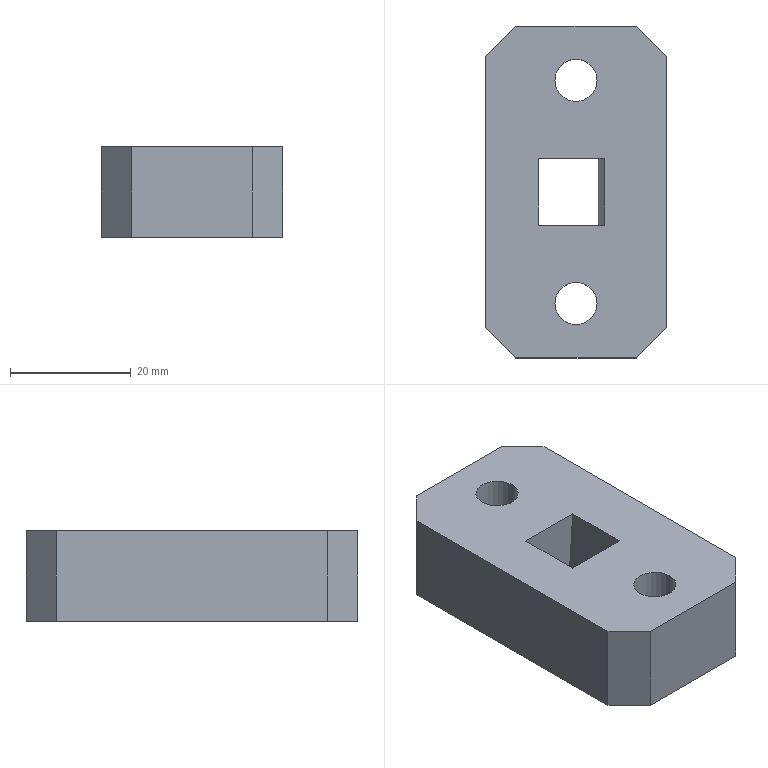Part | Creo | 1 solid | 137 faces | box 30.003 x 55 x 15 mm | volume 20234 mm3 | other 77 | plane 50 | cylinder 10 | commonest cylinder face diameters 7 x4 11 x4 1.421 x1 22.406 x1